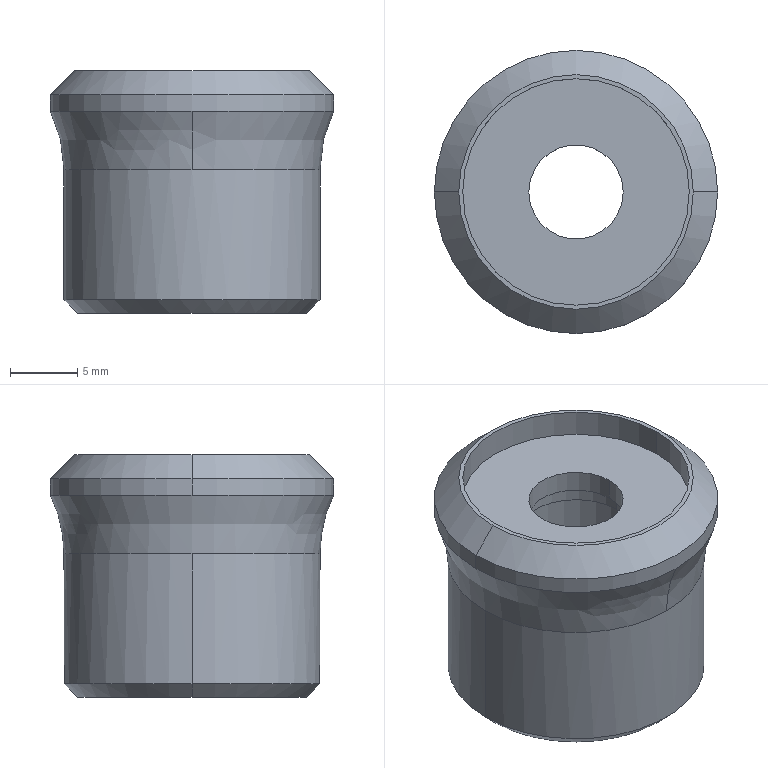Part | SolidWorks | features BaseBody 1 | 1 solid | 27 faces | box 21 x 21 x 18 mm | volume 3629 mm3 | cylinder 14 | cone 6 | plane 5 | spline 2 | commonest cylinder face diameters 7 x2 8.5 x2 10 x2 12.2 x2 16.8 x2 19 x2
STEP:
#1=CARTESIAN_POINT('',(491.037,37.715,100.866));
#2=VERTEX_POINT('',#1);
#3=CARTESIAN_POINT('',(480.537,27.215,100.866));
#4=VERTEX_POINT('',#3);
#5=CARTESIAN_POINT('',(480.537,37.715,100.866));
#6=DIRECTION('',(0.000000013,0.,-1.));
#7=DIRECTION('',(0.,1.,0.));
#8=AXIS2_PLACEMENT_3D('',#5,#6,#7);
#9=CIRCLE('',#8,10.5);
#10=EDGE_CURVE('',#2,#4,#9,.T.);
#11=ORIENTED_EDGE('',*,*,#10,.T.);
#12=CARTESIAN_POINT('',(480.537,28.215,96.507));
#13=VERTEX_POINT('',#12);
#14=CARTESIAN_POINT('',(480.537,27.215,100.866));
#15=CARTESIAN_POINT('',(480.537,27.542,100.189));
#16=CARTESIAN_POINT('',(480.537,28.044,98.762));
#17=CARTESIAN_POINT('',(480.537,28.215,97.259));
#18=CARTESIAN_POINT('',(480.537,28.215,96.507));
#19=B_SPLINE_CURVE_WITH_KNOTS('',3,(#14,#15,#16,#17,#18),.UNSPECIFIED.,.F.,.F.,(4,1,4),(0.01923,0.5,0.9808),.UNSPECIFIED.);
#20=EDGE_CURVE('',#4,#13,#19,.T.);
#21=ORIENTED_EDGE('',*,*,#20,.T.);
#22=CARTESIAN_POINT('',(490.037,37.715,96.507));
#23=VERTEX_POINT('',#22);
#24=CARTESIAN_POINT('',(480.537,37.715,96.507));
#25=DIRECTION('',(-0.000000013,0.,1.));
#26=DIRECTION('',(0.,1.,0.));
#27=AXIS2_PLACEMENT_3D('',#24,#25,#26);
#28=CIRCLE('',#27,9.5);
#29=EDGE_CURVE('',#13,#23,#28,.T.);
#30=ORIENTED_EDGE('',*,*,#29,.T.);
#31=CARTESIAN_POINT('',(480.537,47.215,96.507));
#32=VERTEX_POINT('',#31);
#33=CARTESIAN_POINT('',(480.537,37.715,96.507));
#34=DIRECTION('',(-0.000000013,0.,1.));
#35=DIRECTION('',(0.,1.,0.));
#36=AXIS2_PLACEMENT_3D('',#33,#34,#35);
#37=CIRCLE('',#36,9.5);
#38=EDGE_CURVE('',#23,#32,#37,.T.);
#39=ORIENTED_EDGE('',*,*,#38,.T.);
#40=CARTESIAN_POINT('',(480.537,48.215,100.866));
#41=VERTEX_POINT('',#40);
#42=CARTESIAN_POINT('',(480.537,48.215,100.866));
#43=CARTESIAN_POINT('',(480.537,47.887,100.189));
#44=CARTESIAN_POINT('',(480.537,47.385,98.762));
#45=CARTESIAN_POINT('',(480.537,47.215,97.259));
#46=CARTESIAN_POINT('',(480.537,47.215,96.507));
#47=B_SPLINE_CURVE_WITH_KNOTS('',3,(#42,#43,#44,#45,#46),.UNSPECIFIED.,.F.,.F.,(4,1,4),(0.01923,0.5,0.9808),.UNSPECIFIED.);
#48=EDGE_CURVE('',#41,#32,#47,.T.);
#49=ORIENTED_EDGE('',*,*,#48,.F.);
#50=CARTESIAN_POINT('',(480.537,37.715,100.866));
#51=DIRECTION('',(0.000000013,0.,-1.));
#52=DIRECTION('',(0.,1.,0.));
#53=AXIS2_PLACEMENT_3D('',#50,#51,#52);
#54=CIRCLE('',#53,10.5);
#55=EDGE_CURVE('',#41,#2,#54,.T.);
#56=ORIENTED_EDGE('',*,*,#55,.T.);
#57=EDGE_LOOP('',(#11,#21,#30,#39,#49,#56));
#58=FACE_OUTER_BOUND('',#57,.T.);
#59=CARTESIAN_POINT('',(480.537,27.215,100.866));
#60=CARTESIAN_POINT('',(486.688,27.215,100.866));
#61=CARTESIAN_POINT('',(491.037,31.564,100.866));
#62=CARTESIAN_POINT('',(491.037,37.715,100.866));
#63=CARTESIAN_POINT('',(491.037,43.865,100.866));
#64=CARTESIAN_POINT('',(486.688,48.215,100.866));
#65=CARTESIAN_POINT('',(480.537,48.215,100.866));
#66=CARTESIAN_POINT('',(480.537,27.542,100.189));
#67=CARTESIAN_POINT('',(486.496,27.542,100.189));
#68=CARTESIAN_POINT('',(490.709,31.756,100.189));
#69=CARTESIAN_POINT('',(490.709,37.715,100.189));
#70=CARTESIAN_POINT('',(490.709,43.674,100.189));
#71=CARTESIAN_POINT('',(486.496,47.887,100.189));
#72=CARTESIAN_POINT('',(480.537,47.887,100.189));
#73=CARTESIAN_POINT('',(480.537,28.044,98.762));
#74=CARTESIAN_POINT('',(486.202,28.044,98.762));
#75=CARTESIAN_POINT('',(490.207,32.05,98.762));
#76=CARTESIAN_POINT('',(490.207,37.715,98.762));
#77=CARTESIAN_POINT('',(490.207,43.379,98.762));
#78=CARTESIAN_POINT('',(486.202,47.385,98.762));
#79=CARTESIAN_POINT('',(480.537,47.385,98.762));
#80=CARTESIAN_POINT('',(480.537,28.215,97.259));
#81=CARTESIAN_POINT('',(486.102,28.215,97.259));
#82=CARTESIAN_POINT('',(490.037,32.15,97.259));
#83=CARTESIAN_POINT('',(490.037,37.715,97.259));
#84=CARTESIAN_POINT('',(490.037,43.28,97.259));
#85=CARTESIAN_POINT('',(486.102,47.215,97.259));
#86=CARTESIAN_POINT('',(480.537,47.215,97.259));
#87=CARTESIAN_POINT('',(480.537,28.215,96.507));
#88=CARTESIAN_POINT('',(486.102,28.215,96.507));
#89=CARTESIAN_POINT('',(490.037,32.15,96.507));
#90=CARTESIAN_POINT('',(490.037,37.715,96.507));
#91=CARTESIAN_POINT('',(490.037,43.28,96.507));
#92=CARTESIAN_POINT('',(486.102,47.215,96.507));
#93=CARTESIAN_POINT('',(480.537,47.215,96.507));
#94=(BOUNDED_SURFACE()B_SPLINE_SURFACE(3,3,((#59,#60,#61,#62,#63,#64,#65),(#66,#67,#68,#69,#70,#71,#72),(#73,#74,#75,#76,#77,#78,#79),(#80,#81,#82,#83,#84,#85,#86),(#87,#88,#89,#90,#91,#92,#93)),.UNSPECIFIED.,.F.,.F.,.F.)B_SPLINE_SURFACE_WITH_KNOTS((4,1,4),(4,3,4),(0.01923,0.5,0.9808),(0.,0.5,1.),.UNSPECIFIED.)GEOMETRIC_REPRESENTATION_ITEM()RATIONAL_B_SPLINE_SURFACE(((1.,0.8047,0.8047,1.,0.8047,0.8047,1.),(1.,0.8047,0.8047,1.,0.8047,0.8047,1.),(1.,0.8047,0.8047,1.,0.8047,0.8047,1.),(1.,0.8047,0.8047,1.,0.8047,0.8047,1.),(1.,0.8047,0.8047,1.,0.8047,0.8047,1.)))REPRESENTATION_ITEM('')SURFACE());
#95=ADVANCED_FACE('',(#58),#94,.T.);
#96=CARTESIAN_POINT('',(471.037,37.715,86.866));
#97=VERTEX_POINT('',#96);
#98=CARTESIAN_POINT('',(490.037,37.715,86.866));
#99=VERTEX_POINT('',#98);
#100=CARTESIAN_POINT('',(480.537,37.715,86.866));
#101=DIRECTION('',(0.000000013,0.,-1.));
#102=DIRECTION('',(0.,1.,0.));
#103=AXIS2_PLACEMENT_3D('',#100,#101,#102);
#104=CIRCLE('',#103,9.5);
#105=EDGE_CURVE('',#97,#99,#104,.T.);
#106=ORIENTED_EDGE('',*,*,#105,.F.);
#107=CARTESIAN_POINT('',(471.037,37.715,96.507));
#108=VERTEX_POINT('',#107);
#109=CARTESIAN_POINT('',(471.037,37.715,86.866));
#110=DIRECTION('',(-0.000000013,0.,1.));
#111=VECTOR('',#110,1000.);
#112=LINE('',#109,#111);
#113=EDGE_CURVE('',#97,#108,#112,.T.);
#114=ORIENTED_EDGE('',*,*,#113,.T.);
#115=CARTESIAN_POINT('',(480.537,37.715,96.507));
#116=DIRECTION('',(-0.000000013,0.,1.));
#117=DIRECTION('',(0.,1.,0.));
#118=AXIS2_PLACEMENT_3D('',#115,#116,#117);
#119=CIRCLE('',#118,9.5);
#120=EDGE_CURVE('',#32,#108,#119,.T.);
#121=ORIENTED_EDGE('',*,*,#120,.F.);
#122=ORIENTED_EDGE('',*,*,#38,.F.);
#123=CARTESIAN_POINT('',(490.037,37.715,86.866));
#124=DIRECTION('',(-0.000000013,0.,1.));
#125=VECTOR('',#124,1000.);
#126=LINE('',#123,#125);
#127=EDGE_CURVE('',#99,#23,#126,.T.);
#128=ORIENTED_EDGE('',*,*,#127,.F.);
#129=EDGE_LOOP('',(#106,#114,#121,#122,#128));
#130=FACE_OUTER_BOUND('',#129,.T.);
#131=CARTESIAN_POINT('',(480.537,37.715,86.866));
#132=DIRECTION('',(-0.000000013,0.,1.));
#133=DIRECTION('',(1.,0.,0.000000013));
#134=AXIS2_PLACEMENT_3D('',#131,#132,#133);
#135=CYLINDRICAL_SURFACE('',#134,9.5);
#136=ADVANCED_FACE('',(#130),#135,.T.);
#137=CARTESIAN_POINT('',(472.037,37.715,85.866));
#138=VERTEX_POINT('',#137);
#139=CARTESIAN_POINT('',(489.037,37.715,85.866));
#140=VERTEX_POINT('',#139);
#141=CARTESIAN_POINT('',(480.537,37.715,85.866));
#142=DIRECTION('',(0.000000013,0.,-1.));
#143=DIRECTION('',(1.,0.,0.000000013));
#144=AXIS2_PLACEMENT_3D('',#141,#142,#143);
#145=CIRCLE('',#144,8.5);
#146=EDGE_CURVE('',#138,#140,#145,.T.);
#147=ORIENTED_EDGE('',*,*,#146,.F.);
#148=CARTESIAN_POINT('',(472.037,37.715,85.866));
#149=DIRECTION('',(-0.7071,0.,0.7071));
#150=VECTOR('',#149,1000.);
#151=LINE('',#148,#150);
#152=EDGE_CURVE('',#138,#97,#151,.T.);
#153=ORIENTED_EDGE('',*,*,#152,.T.);
#154=ORIENTED_EDGE('',*,*,#105,.T.);
#155=CARTESIAN_POINT('',(489.037,37.715,85.866));
#156=DIRECTION('',(0.7071,0.,0.7071));
#157=VECTOR('',#156,1000.);
#158=LINE('',#155,#157);
#159=EDGE_CURVE('',#140,#99,#158,.T.);
#160=ORIENTED_EDGE('',*,*,#159,.F.);
#161=EDGE_LOOP('',(#147,#153,#154,#160));
#162=FACE_OUTER_BOUND('',#161,.T.);
#163=CARTESIAN_POINT('',(480.537,37.715,85.866));
#164=DIRECTION('',(-0.000000013,0.,1.));
#165=DIRECTION('',(1.,0.,0.000000013));
#166=AXIS2_PLACEMENT_3D('',#163,#164,#165);
#167=CONICAL_SURFACE('',#166,8.5,0.7854);
#168=ADVANCED_FACE('',(#162),#167,.T.);
#169=CARTESIAN_POINT('',(470.037,37.715,100.866));
#170=VERTEX_POINT('',#169);
#171=CARTESIAN_POINT('',(480.537,37.715,100.866));
#172=DIRECTION('',(0.000000013,0.,-1.));
#173=DIRECTION('',(0.,1.,0.));
#174=AXIS2_PLACEMENT_3D('',#171,#172,#173);
#175=CIRCLE('',#174,10.5);
#176=EDGE_CURVE('',#170,#41,#175,.T.);
#177=ORIENTED_EDGE('',*,*,#176,.F.);
#178=CARTESIAN_POINT('',(470.037,37.715,102.066));
#179=VERTEX_POINT('',#178);
#180=CARTESIAN_POINT('',(470.037,37.715,100.866));
#181=DIRECTION('',(-0.000000013,0.,1.));
#182=VECTOR('',#181,1000.);
#183=LINE('',#180,#182);
#184=EDGE_CURVE('',#170,#179,#183,.T.);
#185=ORIENTED_EDGE('',*,*,#184,.T.);
#186=CARTESIAN_POINT('',(491.037,37.715,102.066));
#187=VERTEX_POINT('',#186);
#188=CARTESIAN_POINT('',(480.537,37.715,102.066));
#189=DIRECTION('',(-0.000000013,0.,1.));
#190=DIRECTION('',(0.,1.,0.));
#191=AXIS2_PLACEMENT_3D('',#188,#189,#190);
#192=CIRCLE('',#191,10.5);
#193=EDGE_CURVE('',#187,#179,#192,.T.);
#194=ORIENTED_EDGE('',*,*,#193,.F.);
#195=CARTESIAN_POINT('',(491.037,37.715,100.866));
#196=DIRECTION('',(-0.000000013,0.,1.));
#197=VECTOR('',#196,1000.);
#198=LINE('',#195,#197);
#199=EDGE_CURVE('',#2,#187,#198,.T.);
#200=ORIENTED_EDGE('',*,*,#199,.F.);
#201=ORIENTED_EDGE('',*,*,#55,.F.);
#202=EDGE_LOOP('',(#177,#185,#194,#200,#201));
#203=FACE_OUTER_BOUND('',#202,.T.);
#204=CARTESIAN_POINT('',(480.537,37.715,100.866));
#205=DIRECTION('',(-0.000000013,0.,1.));
#206=DIRECTION('',(1.,0.,0.000000013));
#207=AXIS2_PLACEMENT_3D('',#204,#205,#206);
#208=CYLINDRICAL_SURFACE('',#207,10.5);
#209=ADVANCED_FACE('',(#203),#208,.T.);
#210=CARTESIAN_POINT('',(489.237,37.715,103.866));
#211=VERTEX_POINT('',#210);
#212=CARTESIAN_POINT('',(471.837,37.715,103.866));
#213=VERTEX_POINT('',#212);
#214=CARTESIAN_POINT('',(480.537,37.715,103.866));
#215=DIRECTION('',(-0.000000013,0.,1.));
#216=DIRECTION('',(-1.,0.,-0.000000013));
#217=AXIS2_PLACEMENT_3D('',#214,#215,#216);
#218=CIRCLE('',#217,8.7);
#219=EDGE_CURVE('',#211,#213,#218,.T.);
#220=ORIENTED_EDGE('',*,*,#219,.F.);
#221=CARTESIAN_POINT('',(491.037,37.715,102.066));
#222=DIRECTION('',(0.7071,0.,-0.7071));
#223=VECTOR('',#222,1000.);
#224=LINE('',#221,#223);
#225=EDGE_CURVE('',#211,#187,#224,.T.);
#226=ORIENTED_EDGE('',*,*,#225,.T.);
#227=ORIENTED_EDGE('',*,*,#193,.T.);
#228=CARTESIAN_POINT('',(470.037,37.715,102.066));
#229=DIRECTION('',(-0.7071,0.,-0.7071));
#230=VECTOR('',#229,1000.);
#231=LINE('',#228,#230);
#232=EDGE_CURVE('',#213,#179,#231,.T.);
#233=ORIENTED_EDGE('',*,*,#232,.F.);
#234=EDGE_LOOP('',(#220,#226,#227,#233));
#235=FACE_OUTER_BOUND('',#234,.T.);
#236=CARTESIAN_POINT('',(480.537,37.715,102.066));
#237=DIRECTION('',(0.000000013,0.,-1.));
#238=DIRECTION('',(-1.,0.,-0.000000013));
#239=AXIS2_PLACEMENT_3D('',#236,#237,#238);
#240=CONICAL_SURFACE('',#239,10.5,0.7854);
#241=ADVANCED_FACE('',(#235),#240,.T.);
#242=CARTESIAN_POINT('',(486.637,37.715,85.866));
#243=VERTEX_POINT('',#242);
#244=CARTESIAN_POINT('',(474.437,37.715,85.866));
#245=VERTEX_POINT('',#244);
#246=CARTESIAN_POINT('',(480.537,37.715,85.866));
#247=DIRECTION('',(0.000000013,0.,-1.));
#248=DIRECTION('',(1.,0.,0.000000013));
#249=AXIS2_PLACEMENT_3D('',#246,#247,#248);
#250=CIRCLE('',#249,6.1);
#251=EDGE_CURVE('',#243,#245,#250,.T.);
#252=ORIENTED_EDGE('',*,*,#251,.T.);
#253=CARTESIAN_POINT('',(474.437,37.715,86.366));
#254=VERTEX_POINT('',#253);
#255=CARTESIAN_POINT('',(474.437,37.715,85.866));
#256=DIRECTION('',(-0.000000013,0.,1.));
#257=VECTOR('',#256,1000.);
#258=LINE('',#255,#257);
#259=EDGE_CURVE('',#245,#254,#258,.T.);
#260=ORIENTED_EDGE('',*,*,#259,.T.);
#261=CARTESIAN_POINT('',(486.637,37.715,86.366));
#262=VERTEX_POINT('',#261);
#263=CARTESIAN_POINT('',(480.537,37.715,86.366));
#264=DIRECTION('',(-0.000000013,0.,1.));
#265=DIRECTION('',(1.,0.,0.000000013));
#266=AXIS2_PLACEMENT_3D('',#263,#264,#265);
#267=CIRCLE('',#266,6.1);
#268=EDGE_CURVE('',#254,#262,#267,.T.);
#269=ORIENTED_EDGE('',*,*,#268,.T.);
#270=CARTESIAN_POINT('',(486.637,37.715,85.866));
#271=DIRECTION('',(-0.000000013,0.,1.));
#272=VECTOR('',#271,1000.);
#273=LINE('',#270,#272);
#274=EDGE_CURVE('',#243,#262,#273,.T.);
#275=ORIENTED_EDGE('',*,*,#274,.F.);
#276=EDGE_LOOP('',(#252,#260,#269,#275));
#277=FACE_OUTER_BOUND('',#276,.T.);
#278=CARTESIAN_POINT('',(480.537,37.715,85.866));
#279=DIRECTION('',(-0.000000013,0.,1.));
#280=DIRECTION('',(1.,0.,0.000000013));
#281=AXIS2_PLACEMENT_3D('',#278,#279,#280);
#282=CYLINDRICAL_SURFACE('',#281,6.1);
#283=ADVANCED_FACE('',(#277),#282,.F.);
#284=CARTESIAN_POINT('',(488.937,37.715,101.866));
#285=VERTEX_POINT('',#284);
#286=CARTESIAN_POINT('',(472.137,37.715,101.866));
#287=VERTEX_POINT('',#286);
#288=CARTESIAN_POINT('',(480.537,37.715,101.866));
#289=DIRECTION('',(0.000000013,0.,-1.));
#290=DIRECTION('',(1.,0.,0.000000013));
#291=AXIS2_PLACEMENT_3D('',#288,#289,#290);
#292=CIRCLE('',#291,8.4);
#293=EDGE_CURVE('',#285,#287,#292,.T.);
#294=ORIENTED_EDGE('',*,*,#293,.T.);
#295=CARTESIAN_POINT('',(472.137,37.715,103.866));
#296=VERTEX_POINT('',#295);
#297=CARTESIAN_POINT('',(472.137,37.715,101.866));
#298=DIRECTION('',(-0.000000013,0.,1.));
#299=VECTOR('',#298,1000.);
#300=LINE('',#297,#299);
#301=EDGE_CURVE('',#287,#296,#300,.T.);
#302=ORIENTED_EDGE('',*,*,#301,.T.);
#303=CARTESIAN_POINT('',(488.937,37.715,103.866));
#304=VERTEX_POINT('',#303);
#305=CARTESIAN_POINT('',(480.537,37.715,103.866));
#306=DIRECTION('',(0.000000013,0.,-1.));
#307=DIRECTION('',(1.,0.,0.000000013));
#308=AXIS2_PLACEMENT_3D('',#305,#306,#307);
#309=CIRCLE('',#308,8.4);
#310=EDGE_CURVE('',#304,#296,#309,.T.);
#311=ORIENTED_EDGE('',*,*,#310,.F.);
#312=CARTESIAN_POINT('',(488.937,37.715,101.866));
#313=DIRECTION('',(-0.000000013,0.,1.));
#314=VECTOR('',#313,1000.);
#315=LINE('',#312,#314);
#316=EDGE_CURVE('',#285,#304,#315,.T.);
#317=ORIENTED_EDGE('',*,*,#316,.F.);
#318=EDGE_LOOP('',(#294,#302,#311,#317));
#319=FACE_OUTER_BOUND('',#318,.T.);
#320=CARTESIAN_POINT('',(480.537,37.715,101.866));
#321=DIRECTION('',(-0.000000013,0.,1.));
#322=DIRECTION('',(1.,0.,0.000000013));
#323=AXIS2_PLACEMENT_3D('',#320,#321,#322);
#324=CYLINDRICAL_SURFACE('',#323,8.4);
#325=ADVANCED_FACE('',(#319),#324,.F.);
#326=CARTESIAN_POINT('',(485.537,37.715,86.366));
#327=VERTEX_POINT('',#326);
#328=CARTESIAN_POINT('',(475.537,37.715,86.366));
#329=VERTEX_POINT('',#328);
#330=CARTESIAN_POINT('',(480.537,37.715,86.366));
#331=DIRECTION('',(0.000000013,0.,-1.));
#332=DIRECTION('',(1.,0.,0.000000013));
#333=AXIS2_PLACEMENT_3D('',#330,#331,#332);
#334=CIRCLE('',#333,5.);
#335=EDGE_CURVE('',#327,#329,#334,.T.);
#336=ORIENTED_EDGE('',*,*,#335,.T.);
#337=CARTESIAN_POINT('',(475.537,37.715,98.866));
#338=VERTEX_POINT('',#337);
#339=CARTESIAN_POINT('',(475.537,37.715,86.366));
#340=DIRECTION('',(-0.000000013,0.,1.));
#341=VECTOR('',#340,1000.);
#342=LINE('',#339,#341);
#343=EDGE_CURVE('',#329,#338,#342,.T.);
#344=ORIENTED_EDGE('',*,*,#343,.T.);
#345=CARTESIAN_POINT('',(485.537,37.715,98.866));
#346=VERTEX_POINT('',#345);
#347=CARTESIAN_POINT('',(480.537,37.715,98.866));
#348=DIRECTION('',(-0.000000013,0.,1.));
#349=DIRECTION('',(1.,0.,0.000000013));
#350=AXIS2_PLACEMENT_3D('',#347,#348,#349);
#351=CIRCLE('',#350,5.);
#352=EDGE_CURVE('',#338,#346,#351,.T.);
#353=ORIENTED_EDGE('',*,*,#352,.T.);
#354=CARTESIAN_POINT('',(485.537,37.715,86.366));
#355=DIRECTION('',(-0.000000013,0.,1.));
#356=VECTOR('',#355,1000.);
#357=LINE('',#354,#356);
#358=EDGE_CURVE('',#327,#346,#357,.T.);
#359=ORIENTED_EDGE('',*,*,#358,.F.);
#360=EDGE_LOOP('',(#336,#344,#353,#359));
#361=FACE_OUTER_BOUND('',#360,.T.);
#362=CARTESIAN_POINT('',(480.537,37.715,86.366));
#363=DIRECTION('',(-0.000000013,0.,1.));
#364=DIRECTION('',(1.,0.,0.000000013));
#365=AXIS2_PLACEMENT_3D('',#362,#363,#364);
#366=CYLINDRICAL_SURFACE('',#365,5.);
#367=ADVANCED_FACE('',(#361),#366,.F.);
#368=CARTESIAN_POINT('',(484.037,37.715,100.265));
#369=VERTEX_POINT('',#368);
#370=CARTESIAN_POINT('',(477.037,37.715,100.265));
#371=VERTEX_POINT('',#370);
#372=CARTESIAN_POINT('',(480.537,37.715,100.265));
#373=DIRECTION('',(0.000000013,0.,-1.));
#374=DIRECTION('',(0.,1.,0.));
#375=AXIS2_PLACEMENT_3D('',#372,#373,#374);
#376=CIRCLE('',#375,3.5);
#377=EDGE_CURVE('',#369,#371,#376,.T.);
#378=ORIENTED_EDGE('',*,*,#377,.T.);
#379=CARTESIAN_POINT('',(477.037,37.715,101.866));
#380=VERTEX_POINT('',#379);
#381=CARTESIAN_POINT('',(477.037,37.715,100.265));
#382=DIRECTION('',(-0.000000013,0.,1.));
#383=VECTOR('',#382,1000.);
#384=LINE('',#381,#383);
#385=EDGE_CURVE('',#371,#380,#384,.T.);
#386=ORIENTED_EDGE('',*,*,#385,.T.);
#387=CARTESIAN_POINT('',(484.037,37.715,101.866));
#388=VERTEX_POINT('',#387);
#389=CARTESIAN_POINT('',(480.537,37.715,101.866));
#390=DIRECTION('',(0.000000013,0.,-1.));
#391=DIRECTION('',(1.,0.,0.000000013));
#392=AXIS2_PLACEMENT_3D('',#389,#390,#391);
#393=CIRCLE('',#392,3.5);
#394=EDGE_CURVE('',#388,#380,#393,.T.);
#395=ORIENTED_EDGE('',*,*,#394,.F.);
#396=CARTESIAN_POINT('',(484.037,37.715,100.265));
#397=DIRECTION('',(-0.000000013,0.,1.));
#398=VECTOR('',#397,1000.);
#399=LINE('',#396,#398);
#400=EDGE_CURVE('',#369,#388,#399,.T.);
#401=ORIENTED_EDGE('',*,*,#400,.F.);
#402=EDGE_LOOP('',(#378,#386,#395,#401));
#403=FACE_OUTER_BOUND('',#402,.T.);
#404=CARTESIAN_POINT('',(480.537,37.715,100.265));
#405=DIRECTION('',(-0.000000013,0.,1.));
#406=DIRECTION('',(1.,0.,0.000000013));
#407=AXIS2_PLACEMENT_3D('',#404,#405,#406);
#408=CYLINDRICAL_SURFACE('',#407,3.5);
#409=ADVANCED_FACE('',(#403),#408,.F.);
#410=CARTESIAN_POINT('',(484.787,37.715,98.866));
#411=VERTEX_POINT('',#410);
#412=CARTESIAN_POINT('',(476.287,37.715,98.866));
#413=VERTEX_POINT('',#412);
#414=CARTESIAN_POINT('',(480.537,37.715,98.866));
#415=DIRECTION('',(0.000000013,0.,-1.));
#416=DIRECTION('',(1.,0.,0.000000013));
#417=AXIS2_PLACEMENT_3D('',#414,#415,#416);
#418=CIRCLE('',#417,4.25);
#419=EDGE_CURVE('',#411,#413,#418,.T.);
#420=ORIENTED_EDGE('',*,*,#419,.T.);
#421=CARTESIAN_POINT('',(476.287,37.715,99.866));
#422=VERTEX_POINT('',#421);
#423=CARTESIAN_POINT('',(476.287,37.715,98.866));
#424=DIRECTION('',(-0.000000013,0.,1.));
#425=VECTOR('',#424,1000.);
#426=LINE('',#423,#425);
#427=EDGE_CURVE('',#413,#422,#426,.T.);
#428=ORIENTED_EDGE('',*,*,#427,.T.);
#429=CARTESIAN_POINT('',(484.787,37.715,99.866));
#430=VERTEX_POINT('',#429);
#431=CARTESIAN_POINT('',(480.537,37.715,99.866));
#432=DIRECTION('',(-0.000000013,0.,1.));
#433=DIRECTION('',(0.,1.,0.));
#434=AXIS2_PLACEMENT_3D('',#431,#432,#433);
#435=CIRCLE('',#434,4.25);
#436=EDGE_CURVE('',#422,#430,#435,.T.);
#437=ORIENTED_EDGE('',*,*,#436,.T.);
#438=CARTESIAN_POINT('',(484.787,37.715,98.866));
#439=DIRECTION('',(-0.000000013,0.,1.));
#440=VECTOR('',#439,1000.);
#441=LINE('',#438,#440);
#442=EDGE_CURVE('',#411,#430,#441,.T.);
#443=ORIENTED_EDGE('',*,*,#442,.F.);
#444=EDGE_LOOP('',(#420,#428,#437,#443));
#445=FACE_OUTER_BOUND('',#444,.T.);
#446=CARTESIAN_POINT('',(480.537,37.715,98.866));
#447=DIRECTION('',(-0.000000013,0.,1.));
#448=DIRECTION('',(1.,0.,0.000000013));
#449=AXIS2_PLACEMENT_3D('',#446,#447,#448);
#450=CYLINDRICAL_SURFACE('',#449,4.25);
#451=ADVANCED_FACE('',(#445),#450,.F.);
#452=ORIENTED_EDGE('',*,*,#377,.F.);
#453=CARTESIAN_POINT('',(484.787,37.715,99.866));
#454=DIRECTION('',(0.8829,0.,-0.4695));
#455=VECTOR('',#454,1000.);
#456=LINE('',#453,#455);
#457=EDGE_CURVE('',#369,#430,#456,.T.);
#458=ORIENTED_EDGE('',*,*,#457,.T.);
#459=ORIENTED_EDGE('',*,*,#436,.F.);
#460=CARTESIAN_POINT('',(476.287,37.715,99.866));
#461=DIRECTION('',(-0.8829,0.,-0.4695));
#462=VECTOR('',#461,1000.);
#463=LINE('',#460,#462);
#464=EDGE_CURVE('',#371,#422,#463,.T.);
#465=ORIENTED_EDGE('',*,*,#464,.F.);
#466=EDGE_LOOP('',(#452,#458,#459,#465));
#467=FACE_OUTER_BOUND('',#466,.T.);
#468=CARTESIAN_POINT('',(480.537,37.715,99.866));
#469=DIRECTION('',(0.000000013,0.,-1.));
#470=DIRECTION('',(-1.,0.,-0.000000013));
#471=AXIS2_PLACEMENT_3D('',#468,#469,#470);
#472=CONICAL_SURFACE('',#471,4.25,1.082);
#473=ADVANCED_FACE('',(#467),#472,.F.);
#474=ORIENTED_EDGE('',*,*,#113,.F.);
#475=CARTESIAN_POINT('',(480.537,37.715,86.866));
#476=DIRECTION('',(0.000000013,0.,-1.));
#477=DIRECTION('',(0.,1.,0.));
#478=AXIS2_PLACEMENT_3D('',#475,#476,#477);
#479=CIRCLE('',#478,9.5);
#480=EDGE_CURVE('',#99,#97,#479,.T.);
#481=ORIENTED_EDGE('',*,*,#480,.F.);
#482=ORIENTED_EDGE('',*,*,#127,.T.);
#483=ORIENTED_EDGE('',*,*,#29,.F.);
#484=CARTESIAN_POINT('',(480.537,37.715,96.507));
#485=DIRECTION('',(-0.000000013,0.,1.));
#486=DIRECTION('',(0.,1.,0.));
#487=AXIS2_PLACEMENT_3D('',#484,#485,#486);
#488=CIRCLE('',#487,9.5);
#489=EDGE_CURVE('',#108,#13,#488,.T.);
#490=ORIENTED_EDGE('',*,*,#489,.F.);
#491=EDGE_LOOP('',(#474,#481,#482,#483,#490));
#492=FACE_OUTER_BOUND('',#491,.T.);
#493=CARTESIAN_POINT('',(480.537,37.715,86.866));
#494=DIRECTION('',(-0.000000013,0.,1.));
#495=DIRECTION('',(1.,0.,0.000000013));
#496=AXIS2_PLACEMENT_3D('',#493,#494,#495);
#497=CYLINDRICAL_SURFACE('',#496,9.5);
#498=ADVANCED_FACE('',(#492),#497,.T.);
#499=ORIENTED_EDGE('',*,*,#20,.F.);
#500=CARTESIAN_POINT('',(480.537,37.715,100.866));
#501=DIRECTION('',(0.000000013,0.,-1.));
#502=DIRECTION('',(0.,1.,0.));
#503=AXIS2_PLACEMENT_3D('',#500,#501,#502);
#504=CIRCLE('',#503,10.5);
#505=EDGE_CURVE('',#4,#170,#504,.T.);
#506=ORIENTED_EDGE('',*,*,#505,.T.);
#507=ORIENTED_EDGE('',*,*,#176,.T.);
#508=ORIENTED_EDGE('',*,*,#48,.T.);
#509=ORIENTED_EDGE('',*,*,#120,.T.);
#510=ORIENTED_EDGE('',*,*,#489,.T.);
#511=EDGE_LOOP('',(#499,#506,#507,#508,#509,#510));
#512=FACE_OUTER_BOUND('',#511,.T.);
#513=CARTESIAN_POINT('',(480.537,48.215,100.866));
#514=CARTESIAN_POINT('',(459.537,48.215,100.866));
#515=CARTESIAN_POINT('',(459.537,27.215,100.866));
#516=CARTESIAN_POINT('',(480.537,27.215,100.866));
#517=CARTESIAN_POINT('',(480.537,47.887,100.189));
#518=CARTESIAN_POINT('',(460.192,47.887,100.189));
#519=CARTESIAN_POINT('',(460.192,27.542,100.189));
#520=CARTESIAN_POINT('',(480.537,27.542,100.189));
#521=CARTESIAN_POINT('',(480.537,47.385,98.762));
#522=CARTESIAN_POINT('',(461.196,47.385,98.762));
#523=CARTESIAN_POINT('',(461.196,28.044,98.762));
#524=CARTESIAN_POINT('',(480.537,28.044,98.762));
#525=CARTESIAN_POINT('',(480.537,47.215,97.259));
#526=CARTESIAN_POINT('',(461.537,47.215,97.259));
#527=CARTESIAN_POINT('',(461.537,28.215,97.259));
#528=CARTESIAN_POINT('',(480.537,28.215,97.259));
#529=CARTESIAN_POINT('',(480.537,47.215,96.507));
#530=CARTESIAN_POINT('',(461.537,47.215,96.507));
#531=CARTESIAN_POINT('',(461.537,28.215,96.507));
#532=CARTESIAN_POINT('',(480.537,28.215,96.507));
#533=(BOUNDED_SURFACE()B_SPLINE_SURFACE(3,3,((#513,#514,#515,#516),(#517,#518,#519,#520),(#521,#522,#523,#524),(#525,#526,#527,#528),(#529,#530,#531,#532)),.UNSPECIFIED.,.F.,.F.,.T.)B_SPLINE_SURFACE_WITH_KNOTS((4,1,4),(4,4),(0.01923,0.5,0.9808),(0.,1.),.UNSPECIFIED.)GEOMETRIC_REPRESENTATION_ITEM()RATIONAL_B_SPLINE_SURFACE(((1.,0.3333,0.3333,1.),(1.,0.3333,0.3333,1.),(1.,0.3333,0.3333,1.),(1.,0.3333,0.3333,1.),(1.,0.3333,0.3333,1.)))REPRESENTATION_ITEM('')SURFACE());
#534=ADVANCED_FACE('',(#512),#533,.T.);
#535=ORIENTED_EDGE('',*,*,#152,.F.);
#536=CARTESIAN_POINT('',(480.537,37.715,85.866));
#537=DIRECTION('',(0.000000013,0.,-1.));
#538=DIRECTION('',(1.,0.,0.000000013));
#539=AXIS2_PLACEMENT_3D('',#536,#537,#538);
#540=CIRCLE('',#539,8.5);
#541=EDGE_CURVE('',#140,#138,#540,.T.);
#542=ORIENTED_EDGE('',*,*,#541,.F.);
#543=ORIENTED_EDGE('',*,*,#159,.T.);
#544=ORIENTED_EDGE('',*,*,#480,.T.);
#545=EDGE_LOOP('',(#535,#542,#543,#544));
#546=FACE_OUTER_BOUND('',#545,.T.);
#547=CARTESIAN_POINT('',(480.537,37.715,85.866));
#548=DIRECTION('',(-0.000000013,0.,1.));
#549=DIRECTION('',(1.,0.,0.000000013));
#550=AXIS2_PLACEMENT_3D('',#547,#548,#549);
#551=CONICAL_SURFACE('',#550,8.5,0.7854);
#552=ADVANCED_FACE('',(#546),#551,.T.);
#553=ORIENTED_EDGE('',*,*,#184,.F.);
#554=ORIENTED_EDGE('',*,*,#505,.F.);
#555=ORIENTED_EDGE('',*,*,#10,.F.);
#556=ORIENTED_EDGE('',*,*,#199,.T.);
#557=CARTESIAN_POINT('',(480.537,37.715,102.066));
#558=DIRECTION('',(-0.000000013,0.,1.));
#559=DIRECTION('',(0.,1.,0.));
#560=AXIS2_PLACEMENT_3D('',#557,#558,#559);
#561=CIRCLE('',#560,10.5);
#562=EDGE_CURVE('',#179,#187,#561,.T.);
#563=ORIENTED_EDGE('',*,*,#562,.F.);
#564=EDGE_LOOP('',(#553,#554,#555,#556,#563));
#565=FACE_OUTER_BOUND('',#564,.T.);
#566=CARTESIAN_POINT('',(480.537,37.715,100.866));
#567=DIRECTION('',(-0.000000013,0.,1.));
#568=DIRECTION('',(1.,0.,0.000000013));
#569=AXIS2_PLACEMENT_3D('',#566,#567,#568);
#570=CYLINDRICAL_SURFACE('',#569,10.5);
#571=ADVANCED_FACE('',(#565),#570,.T.);
#572=ORIENTED_EDGE('',*,*,#251,.F.);
#573=CARTESIAN_POINT('',(480.537,37.715,85.866));
#574=DIRECTION('',(0.000000013,0.,-1.));
#575=DIRECTION('',(1.,0.,0.000000013));
#576=AXIS2_PLACEMENT_3D('',#573,#574,#575);
#577=CIRCLE('',#576,6.1);
#578=EDGE_CURVE('',#245,#243,#577,.T.);
#579=ORIENTED_EDGE('',*,*,#578,.F.);
#580=EDGE_LOOP('',(#572,#579));
#581=FACE_BOUND('',#580,.T.);
#582=ORIENTED_EDGE('',*,*,#541,.T.);
#583=ORIENTED_EDGE('',*,*,#146,.T.);
#584=EDGE_LOOP('',(#582,#583));
#585=FACE_OUTER_BOUND('',#584,.T.);
#586=CARTESIAN_POINT('',(489.383,28.875,85.866));
#587=DIRECTION('',(-0.000000013,0.,1.));
#588=DIRECTION('',(0.,1.,0.));
#589=AXIS2_PLACEMENT_3D('',#586,#587,#588);
#590=PLANE('',#589);
#591=ADVANCED_FACE('',(#581,#585),#590,.F.);
#592=ORIENTED_EDGE('',*,*,#225,.F.);
#593=CARTESIAN_POINT('',(480.537,37.715,103.866));
#594=DIRECTION('',(-0.000000013,0.,1.));
#595=DIRECTION('',(-1.,0.,-0.000000013));
#596=AXIS2_PLACEMENT_3D('',#593,#594,#595);
#597=CIRCLE('',#596,8.7);
#598=EDGE_CURVE('',#213,#211,#597,.T.);
#599=ORIENTED_EDGE('',*,*,#598,.F.);
#600=ORIENTED_EDGE('',*,*,#232,.T.);
#601=ORIENTED_EDGE('',*,*,#562,.T.);
#602=EDGE_LOOP('',(#592,#599,#600,#601));
#603=FACE_OUTER_BOUND('',#602,.T.);
#604=CARTESIAN_POINT('',(480.537,37.715,102.066));
#605=DIRECTION('',(0.000000013,0.,-1.));
#606=DIRECTION('',(-1.,0.,-0.000000013));
#607=AXIS2_PLACEMENT_3D('',#604,#605,#606);
#608=CONICAL_SURFACE('',#607,10.5,0.7854);
#609=ADVANCED_FACE('',(#603),#608,.T.);
#610=ORIENTED_EDGE('',*,*,#259,.F.);
#611=ORIENTED_EDGE('',*,*,#578,.T.);
#612=ORIENTED_EDGE('',*,*,#274,.T.);
#613=CARTESIAN_POINT('',(480.537,37.715,86.366));
#614=DIRECTION('',(-0.000000013,0.,1.));
#615=DIRECTION('',(1.,0.,0.000000013));
#616=AXIS2_PLACEMENT_3D('',#613,#614,#615);
#617=CIRCLE('',#616,6.1);
#618=EDGE_CURVE('',#262,#254,#617,.T.);
#619=ORIENTED_EDGE('',*,*,#618,.T.);
#620=EDGE_LOOP('',(#610,#611,#612,#619));
#621=FACE_OUTER_BOUND('',#620,.T.);
#622=CARTESIAN_POINT('',(480.537,37.715,85.866));
#623=DIRECTION('',(-0.000000013,0.,1.));
#624=DIRECTION('',(1.,0.,0.000000013));
#625=AXIS2_PLACEMENT_3D('',#622,#623,#624);
#626=CYLINDRICAL_SURFACE('',#625,6.1);
#627=ADVANCED_FACE('',(#621),#626,.F.);
#628=ORIENTED_EDGE('',*,*,#310,.T.);
#629=CARTESIAN_POINT('',(480.537,37.715,103.866));
#630=DIRECTION('',(0.000000013,0.,-1.));
#631=DIRECTION('',(1.,0.,0.000000013));
#632=AXIS2_PLACEMENT_3D('',#629,#630,#631);
#633=CIRCLE('',#632,8.4);
#634=EDGE_CURVE('',#296,#304,#633,.T.);
#635=ORIENTED_EDGE('',*,*,#634,.T.);
#636=EDGE_LOOP('',(#628,#635));
#637=FACE_BOUND('',#636,.T.);
#638=ORIENTED_EDGE('',*,*,#598,.T.);
#639=ORIENTED_EDGE('',*,*,#219,.T.);
#640=EDGE_LOOP('',(#638,#639));
#641=FACE_OUTER_BOUND('',#640,.T.);
#642=CARTESIAN_POINT('',(489.591,28.667,103.866));
#643=DIRECTION('',(-0.000000013,0.,1.));
#644=DIRECTION('',(0.,1.,0.));
#645=AXIS2_PLACEMENT_3D('',#642,#643,#644);
#646=PLANE('',#645);
#647=ADVANCED_FACE('',(#637,#641),#646,.T.);
#648=ORIENTED_EDGE('',*,*,#335,.F.);
#649=CARTESIAN_POINT('',(480.537,37.715,86.366));
#650=DIRECTION('',(0.000000013,0.,-1.));
#651=DIRECTION('',(1.,0.,0.000000013));
#652=AXIS2_PLACEMENT_3D('',#649,#650,#651);
#653=CIRCLE('',#652,5.);
#654=EDGE_CURVE('',#329,#327,#653,.T.);
#655=ORIENTED_EDGE('',*,*,#654,.F.);
#656=EDGE_LOOP('',(#648,#655));
#657=FACE_BOUND('',#656,.T.);
#658=ORIENTED_EDGE('',*,*,#618,.F.);
#659=ORIENTED_EDGE('',*,*,#268,.F.);
#660=EDGE_LOOP('',(#658,#659));
#661=FACE_OUTER_BOUND('',#660,.T.);
#662=CARTESIAN_POINT('',(486.886,31.371,86.366));
#663=DIRECTION('',(-0.000000013,0.,1.));
#664=DIRECTION('',(0.,1.,0.));
#665=AXIS2_PLACEMENT_3D('',#662,#663,#664);
#666=PLANE('',#665);
#667=ADVANCED_FACE('',(#657,#661),#666,.F.);
#668=ORIENTED_EDGE('',*,*,#301,.F.);
#669=CARTESIAN_POINT('',(480.537,37.715,101.866));
#670=DIRECTION('',(0.000000013,0.,-1.));
#671=DIRECTION('',(1.,0.,0.000000013));
#672=AXIS2_PLACEMENT_3D('',#669,#670,#671);
#673=CIRCLE('',#672,8.4);
#674=EDGE_CURVE('',#287,#285,#673,.T.);
#675=ORIENTED_EDGE('',*,*,#674,.T.);
#676=ORIENTED_EDGE('',*,*,#316,.T.);
#677=ORIENTED_EDGE('',*,*,#634,.F.);
#678=EDGE_LOOP('',(#668,#675,#676,#677));
#679=FACE_OUTER_BOUND('',#678,.T.);
#680=CARTESIAN_POINT('',(480.537,37.715,101.866));
#681=DIRECTION('',(-0.000000013,0.,1.));
#682=DIRECTION('',(1.,0.,0.000000013));
#683=AXIS2_PLACEMENT_3D('',#680,#681,#682);
#684=CYLINDRICAL_SURFACE('',#683,8.4);
#685=ADVANCED_FACE('',(#679),#684,.F.);
#686=ORIENTED_EDGE('',*,*,#343,.F.);
#687=ORIENTED_EDGE('',*,*,#654,.T.);
#688=ORIENTED_EDGE('',*,*,#358,.T.);
#689=CARTESIAN_POINT('',(480.537,37.715,98.866));
#690=DIRECTION('',(-0.000000013,0.,1.));
#691=DIRECTION('',(1.,0.,0.000000013));
#692=AXIS2_PLACEMENT_3D('',#689,#690,#691);
#693=CIRCLE('',#692,5.);
#694=EDGE_CURVE('',#346,#338,#693,.T.);
#695=ORIENTED_EDGE('',*,*,#694,.T.);
#696=EDGE_LOOP('',(#686,#687,#688,#695));
#697=FACE_OUTER_BOUND('',#696,.T.);
#698=CARTESIAN_POINT('',(480.537,37.715,86.366));
#699=DIRECTION('',(-0.000000013,0.,1.));
#700=DIRECTION('',(1.,0.,0.000000013));
#701=AXIS2_PLACEMENT_3D('',#698,#699,#700);
#702=CYLINDRICAL_SURFACE('',#701,5.);
#703=ADVANCED_FACE('',(#697),#702,.F.);
#704=ORIENTED_EDGE('',*,*,#394,.T.);
#705=CARTESIAN_POINT('',(480.537,37.715,101.866));
#706=DIRECTION('',(0.000000013,0.,-1.));
#707=DIRECTION('',(1.,0.,0.000000013));
#708=AXIS2_PLACEMENT_3D('',#705,#706,#707);
#709=CIRCLE('',#708,3.5);
#710=EDGE_CURVE('',#380,#388,#709,.T.);
#711=ORIENTED_EDGE('',*,*,#710,.T.);
#712=EDGE_LOOP('',(#704,#711));
#713=FACE_BOUND('',#712,.T.);
#714=ORIENTED_EDGE('',*,*,#293,.F.);
#715=ORIENTED_EDGE('',*,*,#674,.F.);
#716=EDGE_LOOP('',(#714,#715));
#717=FACE_OUTER_BOUND('',#716,.T.);
#718=CARTESIAN_POINT('',(489.279,28.979,101.866));
#719=DIRECTION('',(-0.000000013,0.,1.));
#720=DIRECTION('',(0.,1.,0.));
#721=AXIS2_PLACEMENT_3D('',#718,#719,#720);
#722=PLANE('',#721);
#723=ADVANCED_FACE('',(#713,#717),#722,.T.);
#724=ORIENTED_EDGE('',*,*,#419,.F.);
#725=CARTESIAN_POINT('',(480.537,37.715,98.866));
#726=DIRECTION('',(0.000000013,0.,-1.));
#727=DIRECTION('',(1.,0.,0.000000013));
#728=AXIS2_PLACEMENT_3D('',#725,#726,#727);
#729=CIRCLE('',#728,4.25);
#730=EDGE_CURVE('',#413,#411,#729,.T.);
#731=ORIENTED_EDGE('',*,*,#730,.F.);
#732=EDGE_LOOP('',(#724,#731));
#733=FACE_BOUND('',#732,.T.);
#734=ORIENTED_EDGE('',*,*,#694,.F.);
#735=ORIENTED_EDGE('',*,*,#352,.F.);
#736=EDGE_LOOP('',(#734,#735));
#737=FACE_OUTER_BOUND('',#736,.T.);
#738=CARTESIAN_POINT('',(485.737,32.515,98.866));
#739=DIRECTION('',(-0.000000013,0.,1.));
#740=DIRECTION('',(0.,1.,0.));
#741=AXIS2_PLACEMENT_3D('',#738,#739,#740);
#742=PLANE('',#741);
#743=ADVANCED_FACE('',(#733,#737),#742,.F.);
#744=ORIENTED_EDGE('',*,*,#385,.F.);
#745=CARTESIAN_POINT('',(480.537,37.715,100.265));
#746=DIRECTION('',(0.000000013,0.,-1.));
#747=DIRECTION('',(0.,1.,0.));
#748=AXIS2_PLACEMENT_3D('',#745,#746,#747);
#749=CIRCLE('',#748,3.5);
#750=EDGE_CURVE('',#371,#369,#749,.T.);
#751=ORIENTED_EDGE('',*,*,#750,.T.);
#752=ORIENTED_EDGE('',*,*,#400,.T.);
#753=ORIENTED_EDGE('',*,*,#710,.F.);
#754=EDGE_LOOP('',(#744,#751,#752,#753));
#755=FACE_OUTER_BOUND('',#754,.T.);
#756=CARTESIAN_POINT('',(480.537,37.715,100.265));
#757=DIRECTION('',(-0.000000013,0.,1.));
#758=DIRECTION('',(1.,0.,0.000000013));
#759=AXIS2_PLACEMENT_3D('',#756,#757,#758);
#760=CYLINDRICAL_SURFACE('',#759,3.5);
#761=ADVANCED_FACE('',(#755),#760,.F.);
#762=ORIENTED_EDGE('',*,*,#427,.F.);
#763=ORIENTED_EDGE('',*,*,#730,.T.);
#764=ORIENTED_EDGE('',*,*,#442,.T.);
#765=CARTESIAN_POINT('',(480.537,37.715,99.866));
#766=DIRECTION('',(-0.000000013,0.,1.));
#767=DIRECTION('',(0.,1.,0.));
#768=AXIS2_PLACEMENT_3D('',#765,#766,#767);
#769=CIRCLE('',#768,4.25);
#770=EDGE_CURVE('',#430,#422,#769,.T.);
#771=ORIENTED_EDGE('',*,*,#770,.T.);
#772=EDGE_LOOP('',(#762,#763,#764,#771));
#773=FACE_OUTER_BOUND('',#772,.T.);
#774=CARTESIAN_POINT('',(480.537,37.715,98.866));
#775=DIRECTION('',(-0.000000013,0.,1.));
#776=DIRECTION('',(1.,0.,0.000000013));
#777=AXIS2_PLACEMENT_3D('',#774,#775,#776);
#778=CYLINDRICAL_SURFACE('',#777,4.25);
#779=ADVANCED_FACE('',(#773),#778,.F.);
#780=ORIENTED_EDGE('',*,*,#457,.F.);
#781=ORIENTED_EDGE('',*,*,#750,.F.);
#782=ORIENTED_EDGE('',*,*,#464,.T.);
#783=ORIENTED_EDGE('',*,*,#770,.F.);
#784=EDGE_LOOP('',(#780,#781,#782,#783));
#785=FACE_OUTER_BOUND('',#784,.T.);
#786=CARTESIAN_POINT('',(480.537,37.715,99.866));
#787=DIRECTION('',(0.000000013,0.,-1.));
#788=DIRECTION('',(-1.,0.,-0.000000013));
#789=AXIS2_PLACEMENT_3D('',#786,#787,#788);
#790=CONICAL_SURFACE('',#789,4.25,1.082);
#791=ADVANCED_FACE('',(#785),#790,.F.);
#792=CLOSED_SHELL('',(#95,#136,#168,#209,#241,#283,#325,#367,#409,#451,#473,#498,#534,#552,#571,#591,#609,#627,#647,#667,#685,#703,#723,#743,#761,#779,#791));
#793=MANIFOLD_SOLID_BREP('',#792);
#794=CARTESIAN_POINT('',(0.,0.,0.));
#795=DIRECTION('',(0.,0.,1.));
#796=DIRECTION('',(1.,0.,0.));
#797=AXIS2_PLACEMENT_3D('',#794,#795,#796);
#798=(LENGTH_UNIT()NAMED_UNIT(*)SI_UNIT(.MILLI.,.METRE.));
#799=UNCERTAINTY_MEASURE_WITH_UNIT(LENGTH_MEASURE(0.00001),#798,'','');
#800=(NAMED_UNIT(*)PLANE_ANGLE_UNIT()SI_UNIT($,.RADIAN.));
#801=(NAMED_UNIT(*)SI_UNIT($,.STERADIAN.)SOLID_ANGLE_UNIT());
#802=(GEOMETRIC_REPRESENTATION_CONTEXT(3)GLOBAL_UNCERTAINTY_ASSIGNED_CONTEXT((#799))GLOBAL_UNIT_ASSIGNED_CONTEXT((#798,#800,#801))REPRESENTATION_CONTEXT('',''));
#803=ADVANCED_BREP_SHAPE_REPRESENTATION('',(#793,#797),#802);